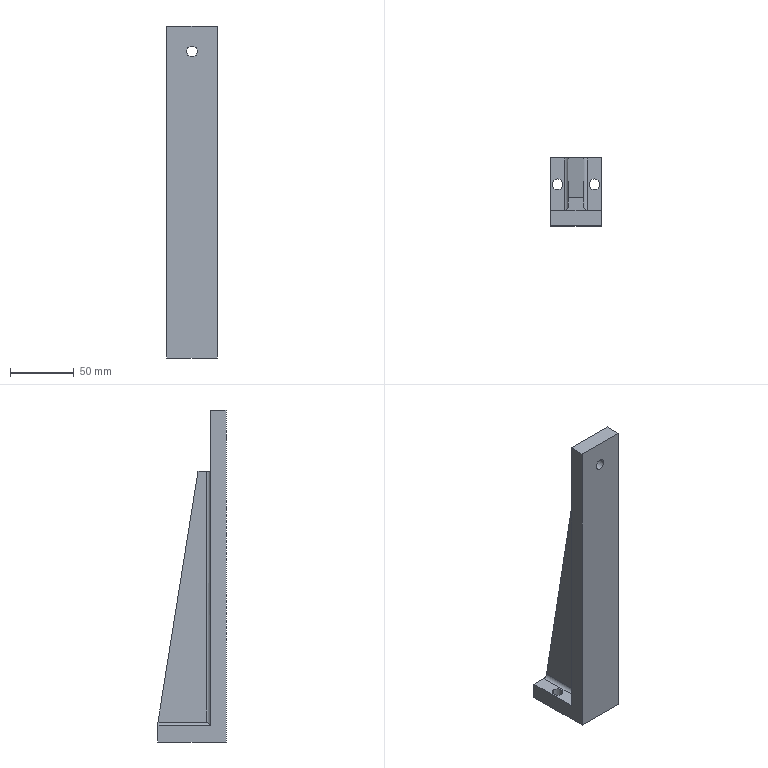Part | STEP file | M10 threaded hole 1-1 | 1 solid | 23 faces | box 40 x 53.4 x 260.669 mm | volume 207154 mm3 | plane 13 | cylinder 10 | commonest cylinder face diameters 8.5 x6 6 x4
STEP:
#1=CARTESIAN_POINT('',(-909.738,-410.823,3118.5));
#2=VERTEX_POINT('',#1);
#3=CARTESIAN_POINT('',(-909.738,-402.323,3118.5));
#4=VERTEX_POINT('',#3);
#5=CARTESIAN_POINT('',(-909.738,-406.573,3118.5));
#6=DIRECTION('',(0.,0.,1.));
#7=DIRECTION('',(0.,1.,0.));
#8=AXIS2_PLACEMENT_3D('',#5,#6,#7);
#9=CIRCLE('',#8,4.25);
#10=EDGE_CURVE('',#2,#4,#9,.T.);
#11=ORIENTED_EDGE('',*,*,#10,.F.);
#12=CARTESIAN_POINT('',(-909.738,-410.823,3131.169));
#13=VERTEX_POINT('',#12);
#14=CARTESIAN_POINT('',(-909.738,-410.823,3131.169));
#15=DIRECTION('',(0.,0.,1.));
#16=VECTOR('',#15,1000.);
#17=LINE('',#14,#16);
#18=EDGE_CURVE('',#2,#13,#17,.T.);
#19=ORIENTED_EDGE('',*,*,#18,.T.);
#20=CARTESIAN_POINT('',(-909.738,-402.323,3131.169));
#21=VERTEX_POINT('',#20);
#22=CARTESIAN_POINT('',(-909.738,-406.573,3131.169));
#23=DIRECTION('',(0.,0.,1.));
#24=DIRECTION('',(0.,1.,0.));
#25=AXIS2_PLACEMENT_3D('',#22,#23,#24);
#26=CIRCLE('',#25,4.25);
#27=EDGE_CURVE('',#13,#21,#26,.T.);
#28=ORIENTED_EDGE('',*,*,#27,.T.);
#29=CARTESIAN_POINT('',(-909.738,-402.323,3131.169));
#30=DIRECTION('',(0.,0.,1.));
#31=VECTOR('',#30,1000.);
#32=LINE('',#29,#31);
#33=EDGE_CURVE('',#4,#21,#32,.T.);
#34=ORIENTED_EDGE('',*,*,#33,.F.);
#35=EDGE_LOOP('',(#11,#19,#28,#34));
#36=FACE_OUTER_BOUND('',#35,.T.);
#37=CARTESIAN_POINT('',(-909.738,-406.573,3131.169));
#38=DIRECTION('',(0.,0.,1.));
#39=DIRECTION('',(0.,-1.,0.));
#40=AXIS2_PLACEMENT_3D('',#37,#38,#39);
#41=CYLINDRICAL_SURFACE('',#40,4.25);
#42=ADVANCED_FACE('',(#36),#41,.F.);
#43=CARTESIAN_POINT('',(-880.738,-410.823,3118.5));
#44=VERTEX_POINT('',#43);
#45=CARTESIAN_POINT('',(-880.738,-402.323,3118.5));
#46=VERTEX_POINT('',#45);
#47=CARTESIAN_POINT('',(-880.738,-406.573,3118.5));
#48=DIRECTION('',(0.,0.,1.));
#49=DIRECTION('',(0.,1.,0.));
#50=AXIS2_PLACEMENT_3D('',#47,#48,#49);
#51=CIRCLE('',#50,4.25);
#52=EDGE_CURVE('',#44,#46,#51,.T.);
#53=ORIENTED_EDGE('',*,*,#52,.F.);
#54=CARTESIAN_POINT('',(-880.738,-410.823,3131.169));
#55=VERTEX_POINT('',#54);
#56=CARTESIAN_POINT('',(-880.738,-410.823,3131.169));
#57=DIRECTION('',(0.,0.,1.));
#58=VECTOR('',#57,1000.);
#59=LINE('',#56,#58);
#60=EDGE_CURVE('',#44,#55,#59,.T.);
#61=ORIENTED_EDGE('',*,*,#60,.T.);
#62=CARTESIAN_POINT('',(-880.738,-402.323,3131.169));
#63=VERTEX_POINT('',#62);
#64=CARTESIAN_POINT('',(-880.738,-406.573,3131.169));
#65=DIRECTION('',(0.,0.,1.));
#66=DIRECTION('',(0.,1.,0.));
#67=AXIS2_PLACEMENT_3D('',#64,#65,#66);
#68=CIRCLE('',#67,4.25);
#69=EDGE_CURVE('',#55,#63,#68,.T.);
#70=ORIENTED_EDGE('',*,*,#69,.T.);
#71=CARTESIAN_POINT('',(-880.738,-402.323,3131.169));
#72=DIRECTION('',(0.,0.,1.));
#73=VECTOR('',#72,1000.);
#74=LINE('',#71,#73);
#75=EDGE_CURVE('',#46,#63,#74,.T.);
#76=ORIENTED_EDGE('',*,*,#75,.F.);
#77=EDGE_LOOP('',(#53,#61,#70,#76));
#78=FACE_OUTER_BOUND('',#77,.T.);
#79=CARTESIAN_POINT('',(-880.738,-406.573,3131.169));
#80=DIRECTION('',(0.,0.,1.));
#81=DIRECTION('',(0.,-1.,0.));
#82=AXIS2_PLACEMENT_3D('',#79,#80,#81);
#83=CYLINDRICAL_SURFACE('',#82,4.25);
#84=ADVANCED_FACE('',(#78),#83,.F.);
#85=CARTESIAN_POINT('',(-890.988,-439.273,3359.169));
#86=VERTEX_POINT('',#85);
#87=CARTESIAN_POINT('',(-899.488,-439.273,3359.169));
#88=VERTEX_POINT('',#87);
#89=CARTESIAN_POINT('',(-895.238,-439.273,3359.169));
#90=DIRECTION('',(0.,1.,0.));
#91=DIRECTION('',(-1.,0.,0.));
#92=AXIS2_PLACEMENT_3D('',#89,#90,#91);
#93=CIRCLE('',#92,4.25);
#94=EDGE_CURVE('',#86,#88,#93,.T.);
#95=ORIENTED_EDGE('',*,*,#94,.F.);
#96=CARTESIAN_POINT('',(-890.988,-427.273,3359.169));
#97=VERTEX_POINT('',#96);
#98=CARTESIAN_POINT('',(-890.988,-427.273,3359.169));
#99=DIRECTION('',(0.,1.,0.));
#100=VECTOR('',#99,1000.);
#101=LINE('',#98,#100);
#102=EDGE_CURVE('',#86,#97,#101,.T.);
#103=ORIENTED_EDGE('',*,*,#102,.T.);
#104=CARTESIAN_POINT('',(-899.488,-427.273,3359.169));
#105=VERTEX_POINT('',#104);
#106=CARTESIAN_POINT('',(-895.238,-427.273,3359.169));
#107=DIRECTION('',(0.,1.,0.));
#108=DIRECTION('',(-1.,0.,0.));
#109=AXIS2_PLACEMENT_3D('',#106,#107,#108);
#110=CIRCLE('',#109,4.25);
#111=EDGE_CURVE('',#97,#105,#110,.T.);
#112=ORIENTED_EDGE('',*,*,#111,.T.);
#113=CARTESIAN_POINT('',(-899.488,-427.273,3359.169));
#114=DIRECTION('',(0.,1.,0.));
#115=VECTOR('',#114,1000.);
#116=LINE('',#113,#115);
#117=EDGE_CURVE('',#88,#105,#116,.T.);
#118=ORIENTED_EDGE('',*,*,#117,.F.);
#119=EDGE_LOOP('',(#95,#103,#112,#118));
#120=FACE_OUTER_BOUND('',#119,.T.);
#121=CARTESIAN_POINT('',(-895.238,-427.273,3359.169));
#122=DIRECTION('',(0.,1.,0.));
#123=DIRECTION('',(1.,0.,0.));
#124=AXIS2_PLACEMENT_3D('',#121,#122,#123);
#125=CYLINDRICAL_SURFACE('',#124,4.25);
#126=ADVANCED_FACE('',(#120),#125,.F.);
#127=CARTESIAN_POINT('',(-880.738,-406.573,3131.169));
#128=DIRECTION('',(0.,0.,1.));
#129=DIRECTION('',(0.,1.,0.));
#130=AXIS2_PLACEMENT_3D('',#127,#128,#129);
#131=CIRCLE('',#130,4.25);
#132=EDGE_CURVE('',#63,#55,#131,.T.);
#133=ORIENTED_EDGE('',*,*,#132,.F.);
#134=ORIENTED_EDGE('',*,*,#69,.F.);
#135=EDGE_LOOP('',(#133,#134));
#136=FACE_BOUND('',#135,.T.);
#137=CARTESIAN_POINT('',(-875.238,-427.273,3131.169));
#138=VERTEX_POINT('',#137);
#139=CARTESIAN_POINT('',(-875.238,-385.874,3131.169));
#140=VERTEX_POINT('',#139);
#141=CARTESIAN_POINT('',(-875.238,-427.273,3131.169));
#142=DIRECTION('',(0.,1.,0.));
#143=VECTOR('',#142,1000.);
#144=LINE('',#141,#143);
#145=EDGE_CURVE('',#138,#140,#144,.T.);
#146=ORIENTED_EDGE('',*,*,#145,.T.);
#147=CARTESIAN_POINT('',(-886.238,-385.874,3131.169));
#148=VERTEX_POINT('',#147);
#149=CARTESIAN_POINT('',(-935.238,-385.874,3131.169));
#150=DIRECTION('',(-1.,0.,0.));
#151=VECTOR('',#150,1000.);
#152=LINE('',#149,#151);
#153=EDGE_CURVE('',#140,#148,#152,.T.);
#154=ORIENTED_EDGE('',*,*,#153,.T.);
#155=CARTESIAN_POINT('',(-886.238,-427.273,3131.169));
#156=VERTEX_POINT('',#155);
#157=CARTESIAN_POINT('',(-886.238,-427.273,3131.169));
#158=DIRECTION('',(0.,-1.,0.));
#159=VECTOR('',#158,1000.);
#160=LINE('',#157,#159);
#161=EDGE_CURVE('',#148,#156,#160,.T.);
#162=ORIENTED_EDGE('',*,*,#161,.T.);
#163=CARTESIAN_POINT('',(-935.238,-427.273,3131.169));
#164=DIRECTION('',(1.,0.,0.));
#165=VECTOR('',#164,1000.);
#166=LINE('',#163,#165);
#167=EDGE_CURVE('',#156,#138,#166,.T.);
#168=ORIENTED_EDGE('',*,*,#167,.T.);
#169=EDGE_LOOP('',(#146,#154,#162,#168));
#170=FACE_OUTER_BOUND('',#169,.T.);
#171=CARTESIAN_POINT('',(-935.238,-427.273,3131.169));
#172=DIRECTION('',(0.,0.,-1.));
#173=DIRECTION('',(1.,0.,0.));
#174=AXIS2_PLACEMENT_3D('',#171,#172,#173);
#175=PLANE('',#174);
#176=ADVANCED_FACE('',(#136,#170),#175,.F.);
#177=CARTESIAN_POINT('',(-895.238,-439.273,3359.169));
#178=DIRECTION('',(0.,1.,0.));
#179=DIRECTION('',(-1.,0.,0.));
#180=AXIS2_PLACEMENT_3D('',#177,#178,#179);
#181=CIRCLE('',#180,4.25);
#182=EDGE_CURVE('',#88,#86,#181,.T.);
#183=ORIENTED_EDGE('',*,*,#182,.T.);
#184=ORIENTED_EDGE('',*,*,#94,.T.);
#185=EDGE_LOOP('',(#183,#184));
#186=FACE_BOUND('',#185,.T.);
#187=CARTESIAN_POINT('',(-915.238,-439.273,3379.169));
#188=VERTEX_POINT('',#187);
#189=CARTESIAN_POINT('',(-915.238,-439.273,3118.5));
#190=VERTEX_POINT('',#189);
#191=CARTESIAN_POINT('',(-915.238,-439.273,3443.5));
#192=DIRECTION('',(0.,0.,-1.));
#193=VECTOR('',#192,1000.);
#194=LINE('',#191,#193);
#195=EDGE_CURVE('',#188,#190,#194,.T.);
#196=ORIENTED_EDGE('',*,*,#195,.T.);
#197=CARTESIAN_POINT('',(-875.238,-439.273,3118.5));
#198=VERTEX_POINT('',#197);
#199=CARTESIAN_POINT('',(-855.238,-439.273,3118.5));
#200=DIRECTION('',(-1.,0.,0.));
#201=VECTOR('',#200,1000.);
#202=LINE('',#199,#201);
#203=EDGE_CURVE('',#198,#190,#202,.T.);
#204=ORIENTED_EDGE('',*,*,#203,.F.);
#205=CARTESIAN_POINT('',(-875.238,-439.273,3379.169));
#206=VERTEX_POINT('',#205);
#207=CARTESIAN_POINT('',(-875.238,-439.273,3443.5));
#208=DIRECTION('',(0.,0.,-1.));
#209=VECTOR('',#208,1000.);
#210=LINE('',#207,#209);
#211=EDGE_CURVE('',#206,#198,#210,.T.);
#212=ORIENTED_EDGE('',*,*,#211,.F.);
#213=CARTESIAN_POINT('',(-855.238,-439.273,3379.169));
#214=DIRECTION('',(-1.,0.,0.));
#215=VECTOR('',#214,1000.);
#216=LINE('',#213,#215);
#217=EDGE_CURVE('',#206,#188,#216,.T.);
#218=ORIENTED_EDGE('',*,*,#217,.T.);
#219=EDGE_LOOP('',(#196,#204,#212,#218));
#220=FACE_OUTER_BOUND('',#219,.T.);
#221=CARTESIAN_POINT('',(-855.238,-439.273,3118.5));
#222=DIRECTION('',(0.,-1.,0.));
#223=DIRECTION('',(-1.,0.,0.));
#224=AXIS2_PLACEMENT_3D('',#221,#222,#223);
#225=PLANE('',#224);
#226=ADVANCED_FACE('',(#186,#220),#225,.T.);
#227=CARTESIAN_POINT('',(-909.738,-406.573,3118.5));
#228=DIRECTION('',(0.,0.,1.));
#229=DIRECTION('',(0.,1.,0.));
#230=AXIS2_PLACEMENT_3D('',#227,#228,#229);
#231=CIRCLE('',#230,4.25);
#232=EDGE_CURVE('',#4,#2,#231,.T.);
#233=ORIENTED_EDGE('',*,*,#232,.T.);
#234=ORIENTED_EDGE('',*,*,#10,.T.);
#235=EDGE_LOOP('',(#233,#234));
#236=FACE_BOUND('',#235,.T.);
#237=CARTESIAN_POINT('',(-880.738,-406.573,3118.5));
#238=DIRECTION('',(0.,0.,1.));
#239=DIRECTION('',(0.,1.,0.));
#240=AXIS2_PLACEMENT_3D('',#237,#238,#239);
#241=CIRCLE('',#240,4.25);
#242=EDGE_CURVE('',#46,#44,#241,.T.);
#243=ORIENTED_EDGE('',*,*,#242,.T.);
#244=ORIENTED_EDGE('',*,*,#52,.T.);
#245=EDGE_LOOP('',(#243,#244));
#246=FACE_BOUND('',#245,.T.);
#247=CARTESIAN_POINT('',(-875.238,-385.874,3118.5));
#248=VERTEX_POINT('',#247);
#249=CARTESIAN_POINT('',(-915.238,-385.874,3118.5));
#250=VERTEX_POINT('',#249);
#251=CARTESIAN_POINT('',(-915.238,-385.874,3118.5));
#252=DIRECTION('',(-1.,0.,0.));
#253=VECTOR('',#252,1000.);
#254=LINE('',#251,#253);
#255=EDGE_CURVE('',#248,#250,#254,.T.);
#256=ORIENTED_EDGE('',*,*,#255,.F.);
#257=CARTESIAN_POINT('',(-875.238,-439.273,3118.5));
#258=DIRECTION('',(0.,1.,0.));
#259=VECTOR('',#258,1000.);
#260=LINE('',#257,#259);
#261=EDGE_CURVE('',#198,#248,#260,.T.);
#262=ORIENTED_EDGE('',*,*,#261,.F.);
#263=ORIENTED_EDGE('',*,*,#203,.T.);
#264=CARTESIAN_POINT('',(-915.238,-439.273,3118.5));
#265=DIRECTION('',(0.,-1.,0.));
#266=VECTOR('',#265,1000.);
#267=LINE('',#264,#266);
#268=EDGE_CURVE('',#250,#190,#267,.T.);
#269=ORIENTED_EDGE('',*,*,#268,.F.);
#270=EDGE_LOOP('',(#256,#262,#263,#269));
#271=FACE_OUTER_BOUND('',#270,.T.);
#272=CARTESIAN_POINT('',(-855.238,-345.874,3118.5));
#273=DIRECTION('',(0.,0.,-1.));
#274=DIRECTION('',(0.,1.,0.));
#275=AXIS2_PLACEMENT_3D('',#272,#273,#274);
#276=PLANE('',#275);
#277=ADVANCED_FACE('',(#236,#246,#271),#276,.T.);
#278=CARTESIAN_POINT('',(-915.238,-427.273,3379.169));
#279=VERTEX_POINT('',#278);
#280=CARTESIAN_POINT('',(-915.238,-439.273,3379.169));
#281=DIRECTION('',(0.,1.,0.));
#282=VECTOR('',#281,1000.);
#283=LINE('',#280,#282);
#284=EDGE_CURVE('',#188,#279,#283,.T.);
#285=ORIENTED_EDGE('',*,*,#284,.F.);
#286=ORIENTED_EDGE('',*,*,#217,.F.);
#287=CARTESIAN_POINT('',(-875.238,-427.273,3379.169));
#288=VERTEX_POINT('',#287);
#289=CARTESIAN_POINT('',(-875.238,-439.273,3379.169));
#290=DIRECTION('',(0.,-1.,0.));
#291=VECTOR('',#290,1000.);
#292=LINE('',#289,#291);
#293=EDGE_CURVE('',#288,#206,#292,.T.);
#294=ORIENTED_EDGE('',*,*,#293,.F.);
#295=CARTESIAN_POINT('',(-935.238,-427.273,3379.169));
#296=DIRECTION('',(1.,0.,0.));
#297=VECTOR('',#296,1000.);
#298=LINE('',#295,#297);
#299=EDGE_CURVE('',#279,#288,#298,.T.);
#300=ORIENTED_EDGE('',*,*,#299,.F.);
#301=EDGE_LOOP('',(#285,#286,#294,#300));
#302=FACE_OUTER_BOUND('',#301,.T.);
#303=CARTESIAN_POINT('',(-855.238,-439.273,3379.169));
#304=DIRECTION('',(0.,0.,1.));
#305=DIRECTION('',(0.,-1.,0.));
#306=AXIS2_PLACEMENT_3D('',#303,#304,#305);
#307=PLANE('',#306);
#308=ADVANCED_FACE('',(#302),#307,.T.);
#309=CARTESIAN_POINT('',(-909.738,-406.573,3131.169));
#310=DIRECTION('',(0.,0.,1.));
#311=DIRECTION('',(0.,1.,0.));
#312=AXIS2_PLACEMENT_3D('',#309,#310,#311);
#313=CIRCLE('',#312,4.25);
#314=EDGE_CURVE('',#21,#13,#313,.T.);
#315=ORIENTED_EDGE('',*,*,#314,.F.);
#316=ORIENTED_EDGE('',*,*,#27,.F.);
#317=EDGE_LOOP('',(#315,#316));
#318=FACE_BOUND('',#317,.T.);
#319=CARTESIAN_POINT('',(-904.238,-427.273,3131.169));
#320=VERTEX_POINT('',#319);
#321=CARTESIAN_POINT('',(-904.238,-385.874,3131.169));
#322=VERTEX_POINT('',#321);
#323=CARTESIAN_POINT('',(-904.238,-354.273,3131.169));
#324=DIRECTION('',(0.,1.,0.));
#325=VECTOR('',#324,1000.);
#326=LINE('',#323,#325);
#327=EDGE_CURVE('',#320,#322,#326,.T.);
#328=ORIENTED_EDGE('',*,*,#327,.T.);
#329=CARTESIAN_POINT('',(-915.238,-385.874,3131.169));
#330=VERTEX_POINT('',#329);
#331=CARTESIAN_POINT('',(-935.238,-385.874,3131.169));
#332=DIRECTION('',(-1.,0.,0.));
#333=VECTOR('',#332,1000.);
#334=LINE('',#331,#333);
#335=EDGE_CURVE('',#322,#330,#334,.T.);
#336=ORIENTED_EDGE('',*,*,#335,.T.);
#337=CARTESIAN_POINT('',(-915.238,-427.273,3131.169));
#338=VERTEX_POINT('',#337);
#339=CARTESIAN_POINT('',(-915.238,-427.273,3131.169));
#340=DIRECTION('',(0.,-1.,0.));
#341=VECTOR('',#340,1000.);
#342=LINE('',#339,#341);
#343=EDGE_CURVE('',#330,#338,#342,.T.);
#344=ORIENTED_EDGE('',*,*,#343,.T.);
#345=CARTESIAN_POINT('',(-935.238,-427.273,3131.169));
#346=DIRECTION('',(1.,0.,0.));
#347=VECTOR('',#346,1000.);
#348=LINE('',#345,#347);
#349=EDGE_CURVE('',#338,#320,#348,.T.);
#350=ORIENTED_EDGE('',*,*,#349,.T.);
#351=EDGE_LOOP('',(#328,#336,#344,#350));
#352=FACE_OUTER_BOUND('',#351,.T.);
#353=CARTESIAN_POINT('',(-935.238,-427.273,3131.169));
#354=DIRECTION('',(0.,0.,-1.));
#355=DIRECTION('',(1.,0.,0.));
#356=AXIS2_PLACEMENT_3D('',#353,#354,#355);
#357=PLANE('',#356);
#358=ADVANCED_FACE('',(#318,#352),#357,.F.);
#359=CARTESIAN_POINT('',(-895.238,-427.273,3359.169));
#360=DIRECTION('',(0.,1.,0.));
#361=DIRECTION('',(-1.,0.,0.));
#362=AXIS2_PLACEMENT_3D('',#359,#360,#361);
#363=CIRCLE('',#362,4.25);
#364=EDGE_CURVE('',#105,#97,#363,.T.);
#365=ORIENTED_EDGE('',*,*,#364,.F.);
#366=ORIENTED_EDGE('',*,*,#111,.F.);
#367=EDGE_LOOP('',(#365,#366));
#368=FACE_BOUND('',#367,.T.);
#369=ORIENTED_EDGE('',*,*,#349,.F.);
#370=CARTESIAN_POINT('',(-915.238,-427.273,3379.169));
#371=DIRECTION('',(0.,0.,1.));
#372=VECTOR('',#371,1000.);
#373=LINE('',#370,#372);
#374=EDGE_CURVE('',#338,#279,#373,.T.);
#375=ORIENTED_EDGE('',*,*,#374,.T.);
#376=ORIENTED_EDGE('',*,*,#299,.T.);
#377=CARTESIAN_POINT('',(-875.238,-427.273,3379.169));
#378=DIRECTION('',(0.,0.,-1.));
#379=VECTOR('',#378,1000.);
#380=LINE('',#377,#379);
#381=EDGE_CURVE('',#288,#138,#380,.T.);
#382=ORIENTED_EDGE('',*,*,#381,.T.);
#383=ORIENTED_EDGE('',*,*,#167,.F.);
#384=CARTESIAN_POINT('',(-886.238,-427.273,3331.169));
#385=VERTEX_POINT('',#384);
#386=CARTESIAN_POINT('',(-886.238,-427.273,3379.169));
#387=DIRECTION('',(0.,0.,1.));
#388=VECTOR('',#387,1000.);
#389=LINE('',#386,#388);
#390=EDGE_CURVE('',#156,#385,#389,.T.);
#391=ORIENTED_EDGE('',*,*,#390,.T.);
#392=CARTESIAN_POINT('',(-904.238,-427.273,3331.169));
#393=VERTEX_POINT('',#392);
#394=CARTESIAN_POINT('',(-935.238,-427.273,3331.169));
#395=DIRECTION('',(-1.,0.,0.));
#396=VECTOR('',#395,1000.);
#397=LINE('',#394,#396);
#398=EDGE_CURVE('',#385,#393,#397,.T.);
#399=ORIENTED_EDGE('',*,*,#398,.T.);
#400=CARTESIAN_POINT('',(-904.238,-427.273,3131.169));
#401=DIRECTION('',(0.,0.,-1.));
#402=VECTOR('',#401,1000.);
#403=LINE('',#400,#402);
#404=EDGE_CURVE('',#393,#320,#403,.T.);
#405=ORIENTED_EDGE('',*,*,#404,.T.);
#406=EDGE_LOOP('',(#369,#375,#376,#382,#383,#391,#399,#405));
#407=FACE_OUTER_BOUND('',#406,.T.);
#408=CARTESIAN_POINT('',(-935.238,-427.273,3379.169));
#409=DIRECTION('',(0.,-1.,0.));
#410=DIRECTION('',(-1.,0.,0.));
#411=AXIS2_PLACEMENT_3D('',#408,#409,#410);
#412=PLANE('',#411);
#413=ADVANCED_FACE('',(#368,#407),#412,.F.);
#414=ORIENTED_EDGE('',*,*,#398,.F.);
#415=CARTESIAN_POINT('',(-889.238,-424.273,3331.169));
#416=VERTEX_POINT('',#415);
#417=CARTESIAN_POINT('',(-886.238,-424.273,3331.169));
#418=DIRECTION('',(0.,0.,-1.));
#419=DIRECTION('',(0.,1.,0.));
#420=AXIS2_PLACEMENT_3D('',#417,#418,#419);
#421=CIRCLE('',#420,3.);
#422=EDGE_CURVE('',#385,#416,#421,.T.);
#423=ORIENTED_EDGE('',*,*,#422,.T.);
#424=CARTESIAN_POINT('',(-889.238,-417.273,3331.169));
#425=VERTEX_POINT('',#424);
#426=CARTESIAN_POINT('',(-889.238,-392.573,3331.169));
#427=DIRECTION('',(0.,-1.,0.));
#428=VECTOR('',#427,1000.);
#429=LINE('',#426,#428);
#430=EDGE_CURVE('',#425,#416,#429,.T.);
#431=ORIENTED_EDGE('',*,*,#430,.F.);
#432=CARTESIAN_POINT('',(-901.238,-417.273,3331.169));
#433=VERTEX_POINT('',#432);
#434=CARTESIAN_POINT('',(-895.238,-417.273,3331.169));
#435=DIRECTION('',(1.,0.,0.));
#436=VECTOR('',#435,1000.);
#437=LINE('',#434,#436);
#438=EDGE_CURVE('',#433,#425,#437,.T.);
#439=ORIENTED_EDGE('',*,*,#438,.F.);
#440=CARTESIAN_POINT('',(-901.238,-424.273,3331.169));
#441=VERTEX_POINT('',#440);
#442=CARTESIAN_POINT('',(-901.238,-392.573,3331.169));
#443=DIRECTION('',(0.,-1.,0.));
#444=VECTOR('',#443,1000.);
#445=LINE('',#442,#444);
#446=EDGE_CURVE('',#433,#441,#445,.T.);
#447=ORIENTED_EDGE('',*,*,#446,.T.);
#448=CARTESIAN_POINT('',(-904.238,-424.273,3331.169));
#449=DIRECTION('',(0.,0.,-1.));
#450=DIRECTION('',(0.,1.,0.));
#451=AXIS2_PLACEMENT_3D('',#448,#449,#450);
#452=CIRCLE('',#451,3.);
#453=EDGE_CURVE('',#441,#393,#452,.T.);
#454=ORIENTED_EDGE('',*,*,#453,.T.);
#455=EDGE_LOOP('',(#414,#423,#431,#439,#447,#454));
#456=FACE_OUTER_BOUND('',#455,.T.);
#457=CARTESIAN_POINT('',(-895.238,-417.273,3331.169));
#458=DIRECTION('',(0.,0.,1.));
#459=DIRECTION('',(0.,1.,0.));
#460=AXIS2_PLACEMENT_3D('',#457,#458,#459);
#461=PLANE('',#460);
#462=ADVANCED_FACE('',(#456),#461,.T.);
#463=CARTESIAN_POINT('',(-889.238,-385.874,3134.169));
#464=VERTEX_POINT('',#463);
#465=CARTESIAN_POINT('',(-889.238,-403.863,3247.035));
#466=DIRECTION('',(0.,0.1574,-0.9875));
#467=VECTOR('',#466,1000.);
#468=LINE('',#465,#467);
#469=EDGE_CURVE('',#425,#464,#468,.T.);
#470=ORIENTED_EDGE('',*,*,#469,.F.);
#471=ORIENTED_EDGE('',*,*,#430,.T.);
#472=CARTESIAN_POINT('',(-889.238,-424.273,3134.169));
#473=VERTEX_POINT('',#472);
#474=CARTESIAN_POINT('',(-889.238,-424.273,3248.835));
#475=DIRECTION('',(0.,0.,-1.));
#476=VECTOR('',#475,1000.);
#477=LINE('',#474,#476);
#478=EDGE_CURVE('',#416,#473,#477,.T.);
#479=ORIENTED_EDGE('',*,*,#478,.T.);
#480=CARTESIAN_POINT('',(-889.238,-392.573,3134.169));
#481=DIRECTION('',(0.,1.,0.));
#482=VECTOR('',#481,1000.);
#483=LINE('',#480,#482);
#484=EDGE_CURVE('',#473,#464,#483,.T.);
#485=ORIENTED_EDGE('',*,*,#484,.T.);
#486=EDGE_LOOP('',(#470,#471,#479,#485));
#487=FACE_OUTER_BOUND('',#486,.T.);
#488=CARTESIAN_POINT('',(-889.238,-392.573,3248.835));
#489=DIRECTION('',(1.,0.,0.));
#490=DIRECTION('',(0.,-1.,0.));
#491=AXIS2_PLACEMENT_3D('',#488,#489,#490);
#492=PLANE('',#491);
#493=ADVANCED_FACE('',(#487),#492,.T.);
#494=ORIENTED_EDGE('',*,*,#446,.F.);
#495=CARTESIAN_POINT('',(-901.238,-385.874,3134.169));
#496=VERTEX_POINT('',#495);
#497=CARTESIAN_POINT('',(-901.238,-417.273,3331.169));
#498=DIRECTION('',(0.,-0.1574,0.9875));
#499=VECTOR('',#498,1000.);
#500=LINE('',#497,#499);
#501=EDGE_CURVE('',#496,#433,#500,.T.);
#502=ORIENTED_EDGE('',*,*,#501,.F.);
#503=CARTESIAN_POINT('',(-901.238,-424.273,3134.169));
#504=VERTEX_POINT('',#503);
#505=CARTESIAN_POINT('',(-901.238,-427.273,3134.169));
#506=DIRECTION('',(0.,-1.,0.));
#507=VECTOR('',#506,1000.);
#508=LINE('',#505,#507);
#509=EDGE_CURVE('',#496,#504,#508,.T.);
#510=ORIENTED_EDGE('',*,*,#509,.T.);
#511=CARTESIAN_POINT('',(-901.238,-424.273,3331.169));
#512=DIRECTION('',(0.,0.,1.));
#513=VECTOR('',#512,1000.);
#514=LINE('',#511,#513);
#515=EDGE_CURVE('',#504,#441,#514,.T.);
#516=ORIENTED_EDGE('',*,*,#515,.T.);
#517=EDGE_LOOP('',(#494,#502,#510,#516));
#518=FACE_OUTER_BOUND('',#517,.T.);
#519=CARTESIAN_POINT('',(-901.238,-392.573,3248.835));
#520=DIRECTION('',(1.,0.,0.));
#521=DIRECTION('',(0.,-1.,0.));
#522=AXIS2_PLACEMENT_3D('',#519,#520,#521);
#523=PLANE('',#522);
#524=ADVANCED_FACE('',(#518),#523,.F.);
#525=ORIENTED_EDGE('',*,*,#161,.F.);
#526=CARTESIAN_POINT('',(-886.238,-385.874,3134.169));
#527=DIRECTION('',(0.,1.,0.));
#528=DIRECTION('',(1.,0.,0.));
#529=AXIS2_PLACEMENT_3D('',#526,#527,#528);
#530=CIRCLE('',#529,3.);
#531=EDGE_CURVE('',#148,#464,#530,.T.);
#532=ORIENTED_EDGE('',*,*,#531,.T.);
#533=ORIENTED_EDGE('',*,*,#484,.F.);
#534=CARTESIAN_POINT('',(-886.238,-427.273,3131.169));
#535=CARTESIAN_POINT('',(-887.996,-427.273,3131.169));
#536=CARTESIAN_POINT('',(-889.238,-426.03,3132.412));
#537=CARTESIAN_POINT('',(-889.238,-424.273,3134.169));
#538=(BOUNDED_CURVE()B_SPLINE_CURVE(3,(#534,#535,#536,#537),.UNSPECIFIED.,.F.,.T.)B_SPLINE_CURVE_WITH_KNOTS((4,4),(0.,1.),.UNSPECIFIED.)CURVE()GEOMETRIC_REPRESENTATION_ITEM()RATIONAL_B_SPLINE_CURVE((1.,0.8047,0.8047,1.))REPRESENTATION_ITEM(''));
#539=EDGE_CURVE('',#156,#473,#538,.T.);
#540=ORIENTED_EDGE('',*,*,#539,.F.);
#541=EDGE_LOOP('',(#525,#532,#533,#540));
#542=FACE_OUTER_BOUND('',#541,.T.);
#543=CARTESIAN_POINT('',(-886.238,-427.273,3134.169));
#544=DIRECTION('',(0.,-1.,0.));
#545=DIRECTION('',(-1.,0.,0.));
#546=AXIS2_PLACEMENT_3D('',#543,#544,#545);
#547=CYLINDRICAL_SURFACE('',#546,3.);
#548=ADVANCED_FACE('',(#542),#547,.F.);
#549=ORIENTED_EDGE('',*,*,#539,.T.);
#550=ORIENTED_EDGE('',*,*,#478,.F.);
#551=ORIENTED_EDGE('',*,*,#422,.F.);
#552=ORIENTED_EDGE('',*,*,#390,.F.);
#553=EDGE_LOOP('',(#549,#550,#551,#552));
#554=FACE_OUTER_BOUND('',#553,.T.);
#555=CARTESIAN_POINT('',(-886.238,-424.273,3379.169));
#556=DIRECTION('',(0.,0.,1.));
#557=DIRECTION('',(0.,-1.,0.));
#558=AXIS2_PLACEMENT_3D('',#555,#556,#557);
#559=CYLINDRICAL_SURFACE('',#558,3.);
#560=ADVANCED_FACE('',(#554),#559,.F.);
#561=ORIENTED_EDGE('',*,*,#453,.F.);
#562=ORIENTED_EDGE('',*,*,#515,.F.);
#563=CARTESIAN_POINT('',(-904.238,-427.273,3131.169));
#564=CARTESIAN_POINT('',(-902.481,-427.273,3131.169));
#565=CARTESIAN_POINT('',(-901.238,-426.03,3132.412));
#566=CARTESIAN_POINT('',(-901.238,-424.273,3134.169));
#567=(BOUNDED_CURVE()B_SPLINE_CURVE(3,(#563,#564,#565,#566),.UNSPECIFIED.,.F.,.T.)B_SPLINE_CURVE_WITH_KNOTS((4,4),(0.,1.),.UNSPECIFIED.)CURVE()GEOMETRIC_REPRESENTATION_ITEM()RATIONAL_B_SPLINE_CURVE((1.,0.8047,0.8047,1.))REPRESENTATION_ITEM(''));
#568=EDGE_CURVE('',#320,#504,#567,.T.);
#569=ORIENTED_EDGE('',*,*,#568,.F.);
#570=ORIENTED_EDGE('',*,*,#404,.F.);
#571=EDGE_LOOP('',(#561,#562,#569,#570));
#572=FACE_OUTER_BOUND('',#571,.T.);
#573=CARTESIAN_POINT('',(-904.238,-424.273,3248.835));
#574=DIRECTION('',(0.,0.,-1.));
#575=DIRECTION('',(0.,1.,0.));
#576=AXIS2_PLACEMENT_3D('',#573,#574,#575);
#577=CYLINDRICAL_SURFACE('',#576,3.);
#578=ADVANCED_FACE('',(#572),#577,.F.);
#579=ORIENTED_EDGE('',*,*,#509,.F.);
#580=CARTESIAN_POINT('',(-904.238,-385.874,3134.169));
#581=DIRECTION('',(0.,1.,0.));
#582=DIRECTION('',(1.,0.,0.));
#583=AXIS2_PLACEMENT_3D('',#580,#581,#582);
#584=CIRCLE('',#583,3.);
#585=EDGE_CURVE('',#496,#322,#584,.T.);
#586=ORIENTED_EDGE('',*,*,#585,.T.);
#587=ORIENTED_EDGE('',*,*,#327,.F.);
#588=ORIENTED_EDGE('',*,*,#568,.T.);
#589=EDGE_LOOP('',(#579,#586,#587,#588));
#590=FACE_OUTER_BOUND('',#589,.T.);
#591=CARTESIAN_POINT('',(-904.238,-392.573,3134.169));
#592=DIRECTION('',(0.,1.,0.));
#593=DIRECTION('',(1.,0.,0.));
#594=AXIS2_PLACEMENT_3D('',#591,#592,#593);
#595=CYLINDRICAL_SURFACE('',#594,3.);
#596=ADVANCED_FACE('',(#590),#595,.F.);
#597=ORIENTED_EDGE('',*,*,#261,.T.);
#598=CARTESIAN_POINT('',(-875.238,-385.874,3443.5));
#599=DIRECTION('',(0.,0.,-1.));
#600=VECTOR('',#599,1000.);
#601=LINE('',#598,#600);
#602=EDGE_CURVE('',#140,#248,#601,.T.);
#603=ORIENTED_EDGE('',*,*,#602,.F.);
#604=ORIENTED_EDGE('',*,*,#145,.F.);
#605=ORIENTED_EDGE('',*,*,#381,.F.);
#606=ORIENTED_EDGE('',*,*,#293,.T.);
#607=ORIENTED_EDGE('',*,*,#211,.T.);
#608=EDGE_LOOP('',(#597,#603,#604,#605,#606,#607));
#609=FACE_OUTER_BOUND('',#608,.T.);
#610=CARTESIAN_POINT('',(-875.238,-439.273,3443.5));
#611=DIRECTION('',(-1.,0.,0.));
#612=DIRECTION('',(0.,1.,0.));
#613=AXIS2_PLACEMENT_3D('',#610,#611,#612);
#614=PLANE('',#613);
#615=ADVANCED_FACE('',(#609),#614,.F.);
#616=ORIENTED_EDGE('',*,*,#343,.F.);
#617=CARTESIAN_POINT('',(-915.238,-385.874,3443.5));
#618=DIRECTION('',(0.,0.,-1.));
#619=VECTOR('',#618,1000.);
#620=LINE('',#617,#619);
#621=EDGE_CURVE('',#330,#250,#620,.T.);
#622=ORIENTED_EDGE('',*,*,#621,.T.);
#623=ORIENTED_EDGE('',*,*,#268,.T.);
#624=ORIENTED_EDGE('',*,*,#195,.F.);
#625=ORIENTED_EDGE('',*,*,#284,.T.);
#626=ORIENTED_EDGE('',*,*,#374,.F.);
#627=EDGE_LOOP('',(#616,#622,#623,#624,#625,#626));
#628=FACE_OUTER_BOUND('',#627,.T.);
#629=CARTESIAN_POINT('',(-915.238,-439.273,3443.5));
#630=DIRECTION('',(1.,0.,0.));
#631=DIRECTION('',(0.,-1.,0.));
#632=AXIS2_PLACEMENT_3D('',#629,#630,#631);
#633=PLANE('',#632);
#634=ADVANCED_FACE('',(#628),#633,.F.);
#635=ORIENTED_EDGE('',*,*,#585,.F.);
#636=CARTESIAN_POINT('',(-915.238,-385.874,3134.169));
#637=DIRECTION('',(1.,0.,0.));
#638=VECTOR('',#637,1000.);
#639=LINE('',#636,#638);
#640=EDGE_CURVE('',#496,#464,#639,.T.);
#641=ORIENTED_EDGE('',*,*,#640,.T.);
#642=ORIENTED_EDGE('',*,*,#531,.F.);
#643=ORIENTED_EDGE('',*,*,#153,.F.);
#644=ORIENTED_EDGE('',*,*,#602,.T.);
#645=ORIENTED_EDGE('',*,*,#255,.T.);
#646=ORIENTED_EDGE('',*,*,#621,.F.);
#647=ORIENTED_EDGE('',*,*,#335,.F.);
#648=EDGE_LOOP('',(#635,#641,#642,#643,#644,#645,#646,#647));
#649=FACE_OUTER_BOUND('',#648,.T.);
#650=CARTESIAN_POINT('',(-915.238,-385.874,3443.5));
#651=DIRECTION('',(0.,-1.,0.));
#652=DIRECTION('',(-1.,0.,0.));
#653=AXIS2_PLACEMENT_3D('',#650,#651,#652);
#654=PLANE('',#653);
#655=ADVANCED_FACE('',(#649),#654,.F.);
#656=ORIENTED_EDGE('',*,*,#469,.T.);
#657=ORIENTED_EDGE('',*,*,#640,.F.);
#658=ORIENTED_EDGE('',*,*,#501,.T.);
#659=ORIENTED_EDGE('',*,*,#438,.T.);
#660=EDGE_LOOP('',(#656,#657,#658,#659));
#661=FACE_OUTER_BOUND('',#660,.T.);
#662=CARTESIAN_POINT('',(-576.238,-417.273,3331.169));
#663=DIRECTION('',(0.,-0.9875,-0.1574));
#664=DIRECTION('',(0.,0.1574,-0.9875));
#665=AXIS2_PLACEMENT_3D('',#662,#663,#664);
#666=PLANE('',#665);
#667=ADVANCED_FACE('',(#661),#666,.F.);
#668=ORIENTED_EDGE('',*,*,#102,.F.);
#669=ORIENTED_EDGE('',*,*,#182,.F.);
#670=ORIENTED_EDGE('',*,*,#117,.T.);
#671=ORIENTED_EDGE('',*,*,#364,.T.);
#672=EDGE_LOOP('',(#668,#669,#670,#671));
#673=FACE_OUTER_BOUND('',#672,.T.);
#674=CARTESIAN_POINT('',(-895.238,-427.273,3359.169));
#675=DIRECTION('',(0.,1.,0.));
#676=DIRECTION('',(1.,0.,0.));
#677=AXIS2_PLACEMENT_3D('',#674,#675,#676);
#678=CYLINDRICAL_SURFACE('',#677,4.25);
#679=ADVANCED_FACE('',(#673),#678,.F.);
#680=ORIENTED_EDGE('',*,*,#60,.F.);
#681=ORIENTED_EDGE('',*,*,#242,.F.);
#682=ORIENTED_EDGE('',*,*,#75,.T.);
#683=ORIENTED_EDGE('',*,*,#132,.T.);
#684=EDGE_LOOP('',(#680,#681,#682,#683));
#685=FACE_OUTER_BOUND('',#684,.T.);
#686=CARTESIAN_POINT('',(-880.738,-406.573,3131.169));
#687=DIRECTION('',(0.,0.,1.));
#688=DIRECTION('',(0.,-1.,0.));
#689=AXIS2_PLACEMENT_3D('',#686,#687,#688);
#690=CYLINDRICAL_SURFACE('',#689,4.25);
#691=ADVANCED_FACE('',(#685),#690,.F.);
#692=ORIENTED_EDGE('',*,*,#18,.F.);
#693=ORIENTED_EDGE('',*,*,#232,.F.);
#694=ORIENTED_EDGE('',*,*,#33,.T.);
#695=ORIENTED_EDGE('',*,*,#314,.T.);
#696=EDGE_LOOP('',(#692,#693,#694,#695));
#697=FACE_OUTER_BOUND('',#696,.T.);
#698=CARTESIAN_POINT('',(-909.738,-406.573,3131.169));
#699=DIRECTION('',(0.,0.,1.));
#700=DIRECTION('',(0.,-1.,0.));
#701=AXIS2_PLACEMENT_3D('',#698,#699,#700);
#702=CYLINDRICAL_SURFACE('',#701,4.25);
#703=ADVANCED_FACE('',(#697),#702,.F.);
#704=CLOSED_SHELL('',(#42,#84,#126,#176,#226,#277,#308,#358,#413,#462,#493,#524,#548,#560,#578,#596,#615,#634,#655,#667,#679,#691,#703));
#705=MANIFOLD_SOLID_BREP('',#704);
#706=CARTESIAN_POINT('',(0.,0.,0.));
#707=DIRECTION('',(0.,0.,1.));
#708=DIRECTION('',(1.,0.,0.));
#709=AXIS2_PLACEMENT_3D('',#706,#707,#708);
#710=(LENGTH_UNIT()NAMED_UNIT(*)SI_UNIT(.MILLI.,.METRE.));
#711=UNCERTAINTY_MEASURE_WITH_UNIT(LENGTH_MEASURE(0.00001),#710,'','');
#712=(NAMED_UNIT(*)PLANE_ANGLE_UNIT()SI_UNIT($,.RADIAN.));
#713=(NAMED_UNIT(*)SI_UNIT($,.STERADIAN.)SOLID_ANGLE_UNIT());
#714=(GEOMETRIC_REPRESENTATION_CONTEXT(3)GLOBAL_UNCERTAINTY_ASSIGNED_CONTEXT((#711))GLOBAL_UNIT_ASSIGNED_CONTEXT((#710,#712,#713))REPRESENTATION_CONTEXT('',''));
#715=ADVANCED_BREP_SHAPE_REPRESENTATION('',(#705,#709),#714);